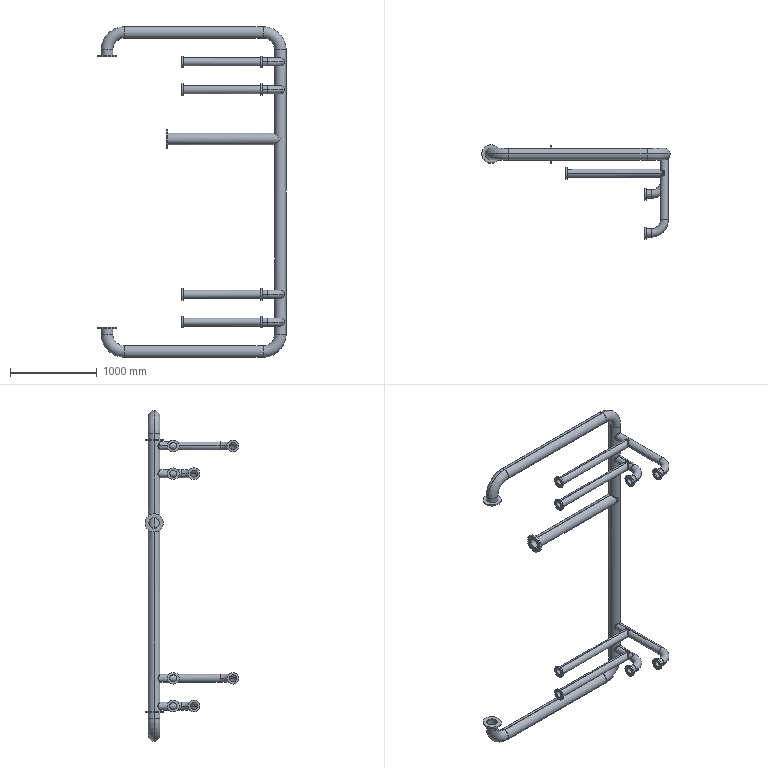Part | SolidWorks | features ICE 9, LPattern 3, Sweep 2 | 1 solid | 226 faces | box 2172 x 1083 x 3813 mm | volume 36791331 mm3 | cylinder 158 | plane 36 | torus 32 | commonest cylinder face diameters 80 x47 92 x47 121 x21 133 x21 135 x16 210 x6